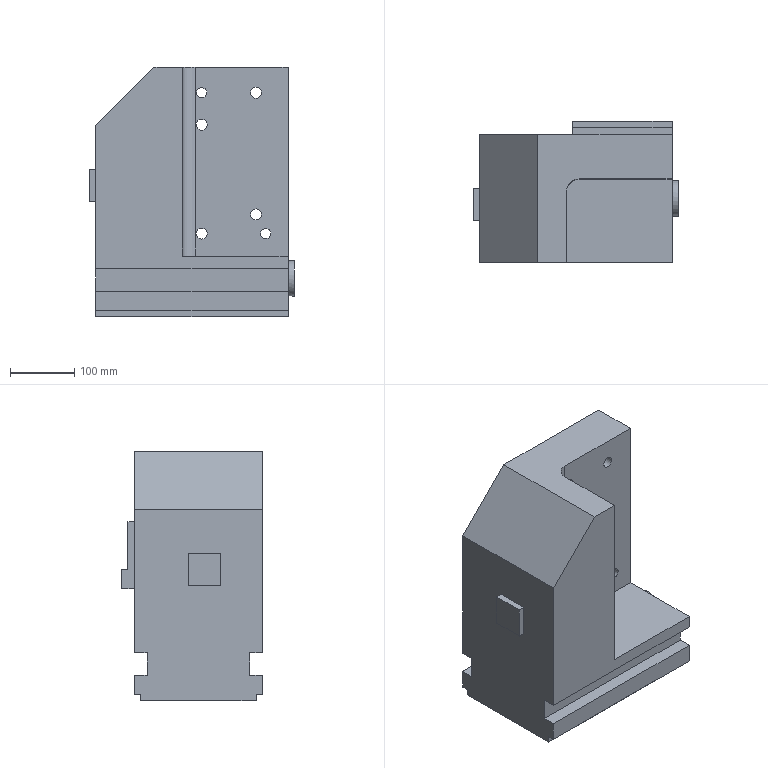Part | NX | features solid 2 | 1 solid | 50 faces | box 320 x 220 x 390 mm | volume 15914614 mm3 | plane 38 | cylinder 12 | commonest cylinder face diameters 17 x4 26 x4 16 x2 40 x1 55 x1
STEP:
#1=CARTESIAN_POINT('',(495.,1030.,-88.));
#2=VERTEX_POINT('',#1);
#3=CARTESIAN_POINT('',(495.,1030.,-75.));
#4=DIRECTION('',(0.,1.,0.));
#5=DIRECTION('',(0.,0.,-1.));
#6=AXIS2_PLACEMENT_3D('',#3,#4,#5);
#7=CIRCLE('',#6,13.);
#8=EDGE_CURVE('',#2,#2,#7,.T.);
#9=ORIENTED_EDGE('',*,*,#8,.F.);
#10=EDGE_LOOP('',(#9));
#11=FACE_BOUND('',#10,.T.);
#12=CARTESIAN_POINT('',(510.,1030.,-97.));
#13=VERTEX_POINT('',#12);
#14=CARTESIAN_POINT('',(510.,1030.,-105.));
#15=DIRECTION('',(0.,1.,0.));
#16=DIRECTION('',(0.,0.,1.));
#17=AXIS2_PLACEMENT_3D('',#14,#15,#16);
#18=CIRCLE('',#17,8.);
#19=EDGE_CURVE('',#13,#13,#18,.F.);
#20=ORIENTED_EDGE('',*,*,#19,.T.);
#21=EDGE_LOOP('',(#20));
#22=FACE_BOUND('',#21,.T.);
#23=CARTESIAN_POINT('',(410.,1030.,-92.));
#24=VERTEX_POINT('',#23);
#25=CARTESIAN_POINT('',(410.,1030.,-105.));
#26=DIRECTION('',(0.,1.,0.));
#27=DIRECTION('',(0.,0.,1.));
#28=AXIS2_PLACEMENT_3D('',#25,#26,#27);
#29=CIRCLE('',#28,13.);
#30=EDGE_CURVE('',#24,#24,#29,.F.);
#31=ORIENTED_EDGE('',*,*,#30,.T.);
#32=EDGE_LOOP('',(#31));
#33=FACE_BOUND('',#32,.T.);
#34=CARTESIAN_POINT('',(495.,1030.,128.));
#35=VERTEX_POINT('',#34);
#36=CARTESIAN_POINT('',(495.,1030.,115.));
#37=DIRECTION('',(0.,1.,0.));
#38=DIRECTION('',(0.,0.,1.));
#39=AXIS2_PLACEMENT_3D('',#36,#37,#38);
#40=CIRCLE('',#39,13.);
#41=EDGE_CURVE('',#35,#35,#40,.F.);
#42=ORIENTED_EDGE('',*,*,#41,.T.);
#43=EDGE_LOOP('',(#42));
#44=FACE_BOUND('',#43,.T.);
#45=CARTESIAN_POINT('',(410.,1030.,123.));
#46=VERTEX_POINT('',#45);
#47=CARTESIAN_POINT('',(410.,1030.,115.));
#48=DIRECTION('',(0.,1.,0.));
#49=DIRECTION('',(0.,0.,1.));
#50=AXIS2_PLACEMENT_3D('',#47,#48,#49);
#51=CIRCLE('',#50,8.);
#52=EDGE_CURVE('',#46,#46,#51,.F.);
#53=ORIENTED_EDGE('',*,*,#52,.T.);
#54=EDGE_LOOP('',(#53));
#55=FACE_BOUND('',#54,.T.);
#56=CARTESIAN_POINT('',(410.,1030.,78.));
#57=VERTEX_POINT('',#56);
#58=CARTESIAN_POINT('',(410.,1030.,65.));
#59=DIRECTION('',(0.,1.,0.));
#60=DIRECTION('',(0.,0.,1.));
#61=AXIS2_PLACEMENT_3D('',#58,#59,#60);
#62=CIRCLE('',#61,13.);
#63=EDGE_CURVE('',#57,#57,#62,.F.);
#64=ORIENTED_EDGE('',*,*,#63,.T.);
#65=EDGE_LOOP('',(#64));
#66=FACE_BOUND('',#65,.T.);
#67=CARTESIAN_POINT('',(390.,1030.,-60.));
#68=VERTEX_POINT('',#67);
#69=CARTESIAN_POINT('',(390.,1030.,45.));
#70=VERTEX_POINT('',#69);
#71=CARTESIAN_POINT('',(390.,1030.,-319.092));
#72=DIRECTION('',(0.,0.,1.));
#73=VECTOR('',#72,1000.);
#74=LINE('',#71,#73);
#75=EDGE_CURVE('',#68,#70,#74,.T.);
#76=ORIENTED_EDGE('',*,*,#75,.F.);
#77=CARTESIAN_POINT('',(545.,1030.,-60.));
#78=VERTEX_POINT('',#77);
#79=CARTESIAN_POINT('',(390.,1030.,-60.));
#80=DIRECTION('',(1.,0.,0.));
#81=VECTOR('',#80,1000.);
#82=LINE('',#79,#81);
#83=EDGE_CURVE('',#68,#78,#82,.T.);
#84=ORIENTED_EDGE('',*,*,#83,.T.);
#85=CARTESIAN_POINT('',(545.,1030.,-160.));
#86=VERTEX_POINT('',#85);
#87=CARTESIAN_POINT('',(545.,1030.,-319.092));
#88=DIRECTION('',(0.,0.,-1.));
#89=VECTOR('',#88,1000.);
#90=LINE('',#87,#89);
#91=EDGE_CURVE('',#86,#78,#90,.F.);
#92=ORIENTED_EDGE('',*,*,#91,.F.);
#93=CARTESIAN_POINT('',(245.,1030.,-160.));
#94=VERTEX_POINT('',#93);
#95=CARTESIAN_POINT('',(319.092,1030.,-160.));
#96=DIRECTION('',(1.,0.,0.));
#97=VECTOR('',#96,1000.);
#98=LINE('',#95,#97);
#99=EDGE_CURVE('',#94,#86,#98,.T.);
#100=ORIENTED_EDGE('',*,*,#99,.F.);
#101=CARTESIAN_POINT('',(245.,1030.,64.411));
#102=VERTEX_POINT('',#101);
#103=CARTESIAN_POINT('',(245.,1030.,0.));
#104=DIRECTION('',(0.,0.,1.));
#105=VECTOR('',#104,1000.);
#106=LINE('',#103,#105);
#107=EDGE_CURVE('',#94,#102,#106,.T.);
#108=ORIENTED_EDGE('',*,*,#107,.T.);
#109=CARTESIAN_POINT('',(335.589,1030.,155.));
#110=VERTEX_POINT('',#109);
#111=CARTESIAN_POINT('',(90.294,1030.,-90.294));
#112=DIRECTION('',(0.7071,0.,0.7071));
#113=VECTOR('',#112,1000.);
#114=LINE('',#111,#113);
#115=EDGE_CURVE('',#102,#110,#114,.T.);
#116=ORIENTED_EDGE('',*,*,#115,.T.);
#117=CARTESIAN_POINT('',(545.,1030.,155.));
#118=VERTEX_POINT('',#117);
#119=CARTESIAN_POINT('',(319.092,1030.,155.));
#120=DIRECTION('',(1.,0.,0.));
#121=VECTOR('',#120,1000.);
#122=LINE('',#119,#121);
#123=EDGE_CURVE('',#110,#118,#122,.T.);
#124=ORIENTED_EDGE('',*,*,#123,.T.);
#125=CARTESIAN_POINT('',(545.,1030.,45.));
#126=VERTEX_POINT('',#125);
#127=CARTESIAN_POINT('',(545.,1030.,-319.092));
#128=DIRECTION('',(0.,0.,-1.));
#129=VECTOR('',#128,1000.);
#130=LINE('',#127,#129);
#131=EDGE_CURVE('',#126,#118,#130,.F.);
#132=ORIENTED_EDGE('',*,*,#131,.F.);
#133=CARTESIAN_POINT('',(390.,1030.,45.));
#134=DIRECTION('',(1.,0.,0.));
#135=VECTOR('',#134,1000.);
#136=LINE('',#133,#135);
#137=EDGE_CURVE('',#70,#126,#136,.T.);
#138=ORIENTED_EDGE('',*,*,#137,.F.);
#139=EDGE_LOOP('',(#76,#84,#92,#100,#108,#116,#124,#132,#138));
#140=FACE_BOUND('',#139,.T.);
#141=CARTESIAN_POINT('',(319.092,1030.,-319.092));
#142=DIRECTION('',(0.,1.,0.));
#143=DIRECTION('',(0.,0.,1.));
#144=AXIS2_PLACEMENT_3D('',#141,#142,#143);
#145=PLANE('',#144);
#146=ADVANCED_FACE('',(#11,#22,#33,#44,#55,#66,#140),#145,.T.);
#147=CARTESIAN_POINT('',(245.,1030.,-225.));
#148=VERTEX_POINT('',#147);
#149=CARTESIAN_POINT('',(245.,1030.,-195.));
#150=VERTEX_POINT('',#149);
#151=CARTESIAN_POINT('',(245.,1030.,0.));
#152=DIRECTION('',(0.,0.,1.));
#153=VECTOR('',#152,1000.);
#154=LINE('',#151,#153);
#155=EDGE_CURVE('',#148,#150,#154,.T.);
#156=ORIENTED_EDGE('',*,*,#155,.T.);
#157=CARTESIAN_POINT('',(545.,1030.,-195.));
#158=VERTEX_POINT('',#157);
#159=CARTESIAN_POINT('',(319.092,1030.,-195.));
#160=DIRECTION('',(1.,0.,0.));
#161=VECTOR('',#160,1000.);
#162=LINE('',#159,#161);
#163=EDGE_CURVE('',#150,#158,#162,.T.);
#164=ORIENTED_EDGE('',*,*,#163,.T.);
#165=CARTESIAN_POINT('',(545.,1030.,-225.));
#166=VERTEX_POINT('',#165);
#167=CARTESIAN_POINT('',(545.,1030.,-319.092));
#168=DIRECTION('',(0.,0.,-1.));
#169=VECTOR('',#168,1000.);
#170=LINE('',#167,#169);
#171=EDGE_CURVE('',#166,#158,#170,.F.);
#172=ORIENTED_EDGE('',*,*,#171,.F.);
#173=CARTESIAN_POINT('',(245.,1030.,-225.));
#174=DIRECTION('',(1.,0.,0.));
#175=VECTOR('',#174,1000.);
#176=LINE('',#173,#175);
#177=EDGE_CURVE('',#148,#166,#176,.T.);
#178=ORIENTED_EDGE('',*,*,#177,.F.);
#179=EDGE_LOOP('',(#156,#164,#172,#178));
#180=FACE_BOUND('',#179,.T.);
#181=CARTESIAN_POINT('',(319.092,1030.,-319.092));
#182=DIRECTION('',(0.,1.,0.));
#183=DIRECTION('',(0.,0.,1.));
#184=AXIS2_PLACEMENT_3D('',#181,#182,#183);
#185=PLANE('',#184);
#186=ADVANCED_FACE('',(#180),#185,.T.);
#187=CARTESIAN_POINT('',(495.,960.,-83.5));
#188=VERTEX_POINT('',#187);
#189=CARTESIAN_POINT('',(495.,960.,-75.));
#190=DIRECTION('',(0.,-1.,0.));
#191=DIRECTION('',(0.,0.,-1.));
#192=AXIS2_PLACEMENT_3D('',#189,#190,#191);
#193=CIRCLE('',#192,8.5);
#194=EDGE_CURVE('',#188,#188,#193,.T.);
#195=ORIENTED_EDGE('',*,*,#194,.F.);
#196=EDGE_LOOP('',(#195));
#197=FACE_BOUND('',#196,.T.);
#198=CARTESIAN_POINT('',(410.,960.,56.5));
#199=VERTEX_POINT('',#198);
#200=CARTESIAN_POINT('',(410.,960.,65.));
#201=DIRECTION('',(0.,-1.,0.));
#202=DIRECTION('',(0.,0.,-1.));
#203=AXIS2_PLACEMENT_3D('',#200,#201,#202);
#204=CIRCLE('',#203,8.5);
#205=EDGE_CURVE('',#199,#199,#204,.T.);
#206=ORIENTED_EDGE('',*,*,#205,.F.);
#207=EDGE_LOOP('',(#206));
#208=FACE_BOUND('',#207,.T.);
#209=CARTESIAN_POINT('',(510.,960.,-113.));
#210=VERTEX_POINT('',#209);
#211=CARTESIAN_POINT('',(510.,960.,-105.));
#212=DIRECTION('',(0.,-1.,0.));
#213=DIRECTION('',(0.,0.,-1.));
#214=AXIS2_PLACEMENT_3D('',#211,#212,#213);
#215=CIRCLE('',#214,8.);
#216=EDGE_CURVE('',#210,#210,#215,.T.);
#217=ORIENTED_EDGE('',*,*,#216,.F.);
#218=EDGE_LOOP('',(#217));
#219=FACE_BOUND('',#218,.T.);
#220=CARTESIAN_POINT('',(410.,960.,-113.5));
#221=VERTEX_POINT('',#220);
#222=CARTESIAN_POINT('',(410.,960.,-105.));
#223=DIRECTION('',(0.,-1.,0.));
#224=DIRECTION('',(0.,0.,-1.));
#225=AXIS2_PLACEMENT_3D('',#222,#223,#224);
#226=CIRCLE('',#225,8.5);
#227=EDGE_CURVE('',#221,#221,#226,.T.);
#228=ORIENTED_EDGE('',*,*,#227,.F.);
#229=EDGE_LOOP('',(#228));
#230=FACE_BOUND('',#229,.T.);
#231=CARTESIAN_POINT('',(545.,960.,-140.));
#232=VERTEX_POINT('',#231);
#233=CARTESIAN_POINT('',(545.,960.,155.));
#234=VERTEX_POINT('',#233);
#235=CARTESIAN_POINT('',(545.,960.,-180.));
#236=DIRECTION('',(0.,0.,-1.));
#237=VECTOR('',#236,1000.);
#238=LINE('',#235,#237);
#239=EDGE_CURVE('',#232,#234,#238,.F.);
#240=ORIENTED_EDGE('',*,*,#239,.T.);
#241=CARTESIAN_POINT('',(400.,960.,155.));
#242=VERTEX_POINT('',#241);
#243=CARTESIAN_POINT('',(472.326,960.,155.));
#244=DIRECTION('',(-1.,0.,0.));
#245=VECTOR('',#244,1000.);
#246=LINE('',#243,#245);
#247=EDGE_CURVE('',#234,#242,#246,.T.);
#248=ORIENTED_EDGE('',*,*,#247,.T.);
#249=CARTESIAN_POINT('',(400.,960.,-140.));
#250=VERTEX_POINT('',#249);
#251=CARTESIAN_POINT('',(400.,960.,-180.));
#252=DIRECTION('',(0.,0.,-1.));
#253=VECTOR('',#252,1000.);
#254=LINE('',#251,#253);
#255=EDGE_CURVE('',#242,#250,#254,.T.);
#256=ORIENTED_EDGE('',*,*,#255,.T.);
#257=CARTESIAN_POINT('',(785.,960.,-140.));
#258=DIRECTION('',(-1.,0.,0.));
#259=VECTOR('',#258,1000.);
#260=LINE('',#257,#259);
#261=EDGE_CURVE('',#250,#232,#260,.F.);
#262=ORIENTED_EDGE('',*,*,#261,.T.);
#263=EDGE_LOOP('',(#240,#248,#256,#262));
#264=FACE_BOUND('',#263,.T.);
#265=CARTESIAN_POINT('',(410.,960.,107.));
#266=VERTEX_POINT('',#265);
#267=CARTESIAN_POINT('',(410.,960.,115.));
#268=DIRECTION('',(0.,-1.,0.));
#269=DIRECTION('',(0.,0.,-1.));
#270=AXIS2_PLACEMENT_3D('',#267,#268,#269);
#271=CIRCLE('',#270,8.);
#272=EDGE_CURVE('',#266,#266,#271,.T.);
#273=ORIENTED_EDGE('',*,*,#272,.F.);
#274=EDGE_LOOP('',(#273));
#275=FACE_BOUND('',#274,.T.);
#276=CARTESIAN_POINT('',(495.,960.,106.5));
#277=VERTEX_POINT('',#276);
#278=CARTESIAN_POINT('',(495.,960.,115.));
#279=DIRECTION('',(0.,-1.,0.));
#280=DIRECTION('',(0.,0.,-1.));
#281=AXIS2_PLACEMENT_3D('',#278,#279,#280);
#282=CIRCLE('',#281,8.5);
#283=EDGE_CURVE('',#277,#277,#282,.T.);
#284=ORIENTED_EDGE('',*,*,#283,.F.);
#285=EDGE_LOOP('',(#284));
#286=FACE_BOUND('',#285,.T.);
#287=CARTESIAN_POINT('',(645.,960.,-180.));
#288=DIRECTION('',(0.,1.,0.));
#289=DIRECTION('',(0.,0.,1.));
#290=AXIS2_PLACEMENT_3D('',#287,#288,#289);
#291=PLANE('',#290);
#292=ADVANCED_FACE('',(#197,#208,#219,#230,#264,#275,#286),#291,.F.);
#293=ORIENTED_EDGE('',*,*,#91,.T.);
#294=CARTESIAN_POINT('',(545.,1050.,-60.));
#295=VERTEX_POINT('',#294);
#296=CARTESIAN_POINT('',(545.,1030.,-60.));
#297=DIRECTION('',(0.,1.,0.));
#298=VECTOR('',#297,1000.);
#299=LINE('',#296,#298);
#300=EDGE_CURVE('',#78,#295,#299,.T.);
#301=ORIENTED_EDGE('',*,*,#300,.T.);
#302=CARTESIAN_POINT('',(545.,1050.,-30.));
#303=VERTEX_POINT('',#302);
#304=CARTESIAN_POINT('',(545.,1050.,-30.));
#305=DIRECTION('',(0.,0.,1.));
#306=VECTOR('',#305,1000.);
#307=LINE('',#304,#306);
#308=EDGE_CURVE('',#303,#295,#307,.F.);
#309=ORIENTED_EDGE('',*,*,#308,.F.);
#310=CARTESIAN_POINT('',(545.,1040.,-30.));
#311=VERTEX_POINT('',#310);
#312=CARTESIAN_POINT('',(545.,1030.,-30.));
#313=DIRECTION('',(0.,1.,0.));
#314=VECTOR('',#313,1000.);
#315=LINE('',#312,#314);
#316=EDGE_CURVE('',#311,#303,#315,.T.);
#317=ORIENTED_EDGE('',*,*,#316,.F.);
#318=CARTESIAN_POINT('',(545.,1040.,45.));
#319=VERTEX_POINT('',#318);
#320=CARTESIAN_POINT('',(545.,1040.,7.5));
#321=DIRECTION('',(0.,0.,1.));
#322=VECTOR('',#321,1000.);
#323=LINE('',#320,#322);
#324=EDGE_CURVE('',#311,#319,#323,.T.);
#325=ORIENTED_EDGE('',*,*,#324,.T.);
#326=CARTESIAN_POINT('',(545.,1035.,45.));
#327=DIRECTION('',(0.,-1.,0.));
#328=VECTOR('',#327,1000.);
#329=LINE('',#326,#328);
#330=EDGE_CURVE('',#319,#126,#329,.T.);
#331=ORIENTED_EDGE('',*,*,#330,.T.);
#332=ORIENTED_EDGE('',*,*,#131,.T.);
#333=CARTESIAN_POINT('',(545.,965.,155.));
#334=DIRECTION('',(0.,-1.,0.));
#335=VECTOR('',#334,1000.);
#336=LINE('',#333,#335);
#337=EDGE_CURVE('',#234,#118,#336,.F.);
#338=ORIENTED_EDGE('',*,*,#337,.F.);
#339=ORIENTED_EDGE('',*,*,#239,.F.);
#340=CARTESIAN_POINT('',(545.,830.,-140.));
#341=VERTEX_POINT('',#340);
#342=CARTESIAN_POINT('',(545.,965.,-140.));
#343=DIRECTION('',(0.,-1.,0.));
#344=VECTOR('',#343,1000.);
#345=LINE('',#342,#344);
#346=EDGE_CURVE('',#232,#341,#345,.T.);
#347=ORIENTED_EDGE('',*,*,#346,.T.);
#348=CARTESIAN_POINT('',(545.,830.,-160.));
#349=VERTEX_POINT('',#348);
#350=CARTESIAN_POINT('',(545.,830.,87.071));
#351=DIRECTION('',(0.,0.,1.));
#352=VECTOR('',#351,1000.);
#353=LINE('',#350,#352);
#354=EDGE_CURVE('',#341,#349,#353,.F.);
#355=ORIENTED_EDGE('',*,*,#354,.T.);
#356=CARTESIAN_POINT('',(545.,850.,-160.));
#357=VERTEX_POINT('',#356);
#358=CARTESIAN_POINT('',(545.,766.,-160.));
#359=DIRECTION('',(0.,-1.,0.));
#360=VECTOR('',#359,1000.);
#361=LINE('',#358,#360);
#362=EDGE_CURVE('',#357,#349,#361,.T.);
#363=ORIENTED_EDGE('',*,*,#362,.F.);
#364=CARTESIAN_POINT('',(545.,850.,-195.));
#365=VERTEX_POINT('',#364);
#366=CARTESIAN_POINT('',(545.,850.,-10.));
#367=DIRECTION('',(0.,0.,-1.));
#368=VECTOR('',#367,1000.);
#369=LINE('',#366,#368);
#370=EDGE_CURVE('',#365,#357,#369,.F.);
#371=ORIENTED_EDGE('',*,*,#370,.F.);
#372=CARTESIAN_POINT('',(545.,830.,-195.));
#373=VERTEX_POINT('',#372);
#374=CARTESIAN_POINT('',(545.,766.,-195.));
#375=DIRECTION('',(0.,-1.,0.));
#376=VECTOR('',#375,1000.);
#377=LINE('',#374,#376);
#378=EDGE_CURVE('',#365,#373,#377,.T.);
#379=ORIENTED_EDGE('',*,*,#378,.T.);
#380=CARTESIAN_POINT('',(545.,830.,-225.));
#381=VERTEX_POINT('',#380);
#382=CARTESIAN_POINT('',(545.,830.,87.071));
#383=DIRECTION('',(0.,0.,1.));
#384=VECTOR('',#383,1000.);
#385=LINE('',#382,#384);
#386=EDGE_CURVE('',#373,#381,#385,.F.);
#387=ORIENTED_EDGE('',*,*,#386,.T.);
#388=CARTESIAN_POINT('',(545.,840.,-225.));
#389=VERTEX_POINT('',#388);
#390=CARTESIAN_POINT('',(545.,830.,-225.));
#391=DIRECTION('',(0.,-1.,0.));
#392=VECTOR('',#391,1000.);
#393=LINE('',#390,#392);
#394=EDGE_CURVE('',#381,#389,#393,.F.);
#395=ORIENTED_EDGE('',*,*,#394,.T.);
#396=CARTESIAN_POINT('',(545.,840.,-235.));
#397=VERTEX_POINT('',#396);
#398=CARTESIAN_POINT('',(545.,840.,-235.));
#399=DIRECTION('',(0.,0.,-1.));
#400=VECTOR('',#399,1000.);
#401=LINE('',#398,#400);
#402=EDGE_CURVE('',#397,#389,#401,.F.);
#403=ORIENTED_EDGE('',*,*,#402,.F.);
#404=CARTESIAN_POINT('',(545.,1020.,-235.));
#405=VERTEX_POINT('',#404);
#406=CARTESIAN_POINT('',(545.,1020.,-235.));
#407=DIRECTION('',(0.,-1.,0.));
#408=VECTOR('',#407,1000.);
#409=LINE('',#406,#408);
#410=EDGE_CURVE('',#397,#405,#409,.F.);
#411=ORIENTED_EDGE('',*,*,#410,.T.);
#412=CARTESIAN_POINT('',(545.,1020.,-225.));
#413=VERTEX_POINT('',#412);
#414=CARTESIAN_POINT('',(545.,1020.,-235.));
#415=DIRECTION('',(0.,0.,-1.));
#416=VECTOR('',#415,1000.);
#417=LINE('',#414,#416);
#418=EDGE_CURVE('',#405,#413,#417,.F.);
#419=ORIENTED_EDGE('',*,*,#418,.T.);
#420=CARTESIAN_POINT('',(545.,1030.,-225.));
#421=DIRECTION('',(0.,-1.,0.));
#422=VECTOR('',#421,1000.);
#423=LINE('',#420,#422);
#424=EDGE_CURVE('',#166,#413,#423,.T.);
#425=ORIENTED_EDGE('',*,*,#424,.F.);
#426=ORIENTED_EDGE('',*,*,#171,.T.);
#427=CARTESIAN_POINT('',(545.,1010.,-195.));
#428=VERTEX_POINT('',#427);
#429=CARTESIAN_POINT('',(545.,1040.,-195.));
#430=DIRECTION('',(0.,-1.,0.));
#431=VECTOR('',#430,1000.);
#432=LINE('',#429,#431);
#433=EDGE_CURVE('',#158,#428,#432,.T.);
#434=ORIENTED_EDGE('',*,*,#433,.T.);
#435=CARTESIAN_POINT('',(545.,1010.,-160.));
#436=VERTEX_POINT('',#435);
#437=CARTESIAN_POINT('',(545.,1010.,-10.));
#438=DIRECTION('',(0.,0.,-1.));
#439=VECTOR('',#438,1000.);
#440=LINE('',#437,#439);
#441=EDGE_CURVE('',#428,#436,#440,.F.);
#442=ORIENTED_EDGE('',*,*,#441,.T.);
#443=CARTESIAN_POINT('',(545.,1040.,-160.));
#444=DIRECTION('',(0.,-1.,0.));
#445=VECTOR('',#444,1000.);
#446=LINE('',#443,#445);
#447=EDGE_CURVE('',#86,#436,#446,.T.);
#448=ORIENTED_EDGE('',*,*,#447,.F.);
#449=EDGE_LOOP('',(#293,#301,#309,#317,#325,#331,#332,#338,#339,#347,#355,#363,#371,#379,#387,#395,#403,#411,#419,#425,#426,#434,#442,#448));
#450=FACE_BOUND('',#449,.T.);
#451=CARTESIAN_POINT('',(545.,957.5,-175.));
#452=VERTEX_POINT('',#451);
#453=CARTESIAN_POINT('',(545.,930.,-175.));
#454=DIRECTION('',(1.,0.,0.));
#455=DIRECTION('',(0.,1.,0.));
#456=AXIS2_PLACEMENT_3D('',#453,#454,#455);
#457=CIRCLE('',#456,27.5);
#458=EDGE_CURVE('',#452,#452,#457,.T.);
#459=ORIENTED_EDGE('',*,*,#458,.F.);
#460=EDGE_LOOP('',(#459));
#461=FACE_BOUND('',#460,.T.);
#462=CARTESIAN_POINT('',(545.,965.,-10.));
#463=DIRECTION('',(1.,0.,0.));
#464=DIRECTION('',(0.,1.,0.));
#465=AXIS2_PLACEMENT_3D('',#462,#463,#464);
#466=PLANE('',#465);
#467=ADVANCED_FACE('',(#450,#461),#466,.T.);
#468=CARTESIAN_POINT('',(245.,1010.,-160.));
#469=VERTEX_POINT('',#468);
#470=CARTESIAN_POINT('',(245.,1040.,-160.));
#471=DIRECTION('',(0.,-1.,0.));
#472=VECTOR('',#471,1000.);
#473=LINE('',#470,#472);
#474=EDGE_CURVE('',#94,#469,#473,.T.);
#475=ORIENTED_EDGE('',*,*,#474,.T.);
#476=CARTESIAN_POINT('',(245.,1010.,-195.));
#477=VERTEX_POINT('',#476);
#478=CARTESIAN_POINT('',(245.,1010.,0.));
#479=DIRECTION('',(0.,0.,1.));
#480=VECTOR('',#479,1000.);
#481=LINE('',#478,#480);
#482=EDGE_CURVE('',#477,#469,#481,.T.);
#483=ORIENTED_EDGE('',*,*,#482,.F.);
#484=CARTESIAN_POINT('',(245.,1040.,-195.));
#485=DIRECTION('',(0.,-1.,0.));
#486=VECTOR('',#485,1000.);
#487=LINE('',#484,#486);
#488=EDGE_CURVE('',#150,#477,#487,.T.);
#489=ORIENTED_EDGE('',*,*,#488,.F.);
#490=ORIENTED_EDGE('',*,*,#155,.F.);
#491=CARTESIAN_POINT('',(245.,1020.,-225.));
#492=VERTEX_POINT('',#491);
#493=CARTESIAN_POINT('',(245.,1030.,-225.));
#494=DIRECTION('',(0.,-1.,0.));
#495=VECTOR('',#494,1000.);
#496=LINE('',#493,#495);
#497=EDGE_CURVE('',#148,#492,#496,.T.);
#498=ORIENTED_EDGE('',*,*,#497,.T.);
#499=CARTESIAN_POINT('',(245.,1020.,-235.));
#500=VERTEX_POINT('',#499);
#501=CARTESIAN_POINT('',(245.,1020.,-235.));
#502=DIRECTION('',(0.,0.,-1.));
#503=VECTOR('',#502,1000.);
#504=LINE('',#501,#503);
#505=EDGE_CURVE('',#500,#492,#504,.F.);
#506=ORIENTED_EDGE('',*,*,#505,.F.);
#507=CARTESIAN_POINT('',(245.,840.,-235.));
#508=VERTEX_POINT('',#507);
#509=CARTESIAN_POINT('',(245.,1020.,-235.));
#510=DIRECTION('',(0.,-1.,0.));
#511=VECTOR('',#510,1000.);
#512=LINE('',#509,#511);
#513=EDGE_CURVE('',#508,#500,#512,.F.);
#514=ORIENTED_EDGE('',*,*,#513,.F.);
#515=CARTESIAN_POINT('',(245.,840.,-225.));
#516=VERTEX_POINT('',#515);
#517=CARTESIAN_POINT('',(245.,840.,-235.));
#518=DIRECTION('',(0.,0.,-1.));
#519=VECTOR('',#518,1000.);
#520=LINE('',#517,#519);
#521=EDGE_CURVE('',#508,#516,#520,.F.);
#522=ORIENTED_EDGE('',*,*,#521,.T.);
#523=CARTESIAN_POINT('',(245.,830.,-225.));
#524=VERTEX_POINT('',#523);
#525=CARTESIAN_POINT('',(245.,830.,-225.));
#526=DIRECTION('',(0.,-1.,0.));
#527=VECTOR('',#526,1000.);
#528=LINE('',#525,#527);
#529=EDGE_CURVE('',#524,#516,#528,.F.);
#530=ORIENTED_EDGE('',*,*,#529,.F.);
#531=CARTESIAN_POINT('',(245.,830.,-195.));
#532=VERTEX_POINT('',#531);
#533=CARTESIAN_POINT('',(245.,830.,0.));
#534=DIRECTION('',(0.,0.,1.));
#535=VECTOR('',#534,1000.);
#536=LINE('',#533,#535);
#537=EDGE_CURVE('',#524,#532,#536,.T.);
#538=ORIENTED_EDGE('',*,*,#537,.T.);
#539=CARTESIAN_POINT('',(245.,850.,-195.));
#540=VERTEX_POINT('',#539);
#541=CARTESIAN_POINT('',(245.,766.,-195.));
#542=DIRECTION('',(0.,1.,0.));
#543=VECTOR('',#542,1000.);
#544=LINE('',#541,#543);
#545=EDGE_CURVE('',#532,#540,#544,.T.);
#546=ORIENTED_EDGE('',*,*,#545,.T.);
#547=CARTESIAN_POINT('',(245.,850.,-160.));
#548=VERTEX_POINT('',#547);
#549=CARTESIAN_POINT('',(245.,850.,0.));
#550=DIRECTION('',(0.,0.,1.));
#551=VECTOR('',#550,1000.);
#552=LINE('',#549,#551);
#553=EDGE_CURVE('',#540,#548,#552,.T.);
#554=ORIENTED_EDGE('',*,*,#553,.T.);
#555=CARTESIAN_POINT('',(245.,830.,-160.));
#556=VERTEX_POINT('',#555);
#557=CARTESIAN_POINT('',(245.,766.,-160.));
#558=DIRECTION('',(0.,1.,0.));
#559=VECTOR('',#558,1000.);
#560=LINE('',#557,#559);
#561=EDGE_CURVE('',#556,#548,#560,.T.);
#562=ORIENTED_EDGE('',*,*,#561,.F.);
#563=CARTESIAN_POINT('',(245.,830.,64.411));
#564=VERTEX_POINT('',#563);
#565=CARTESIAN_POINT('',(245.,830.,0.));
#566=DIRECTION('',(0.,0.,1.));
#567=VECTOR('',#566,1000.);
#568=LINE('',#565,#567);
#569=EDGE_CURVE('',#556,#564,#568,.T.);
#570=ORIENTED_EDGE('',*,*,#569,.T.);
#571=CARTESIAN_POINT('',(245.,0.,64.411));
#572=DIRECTION('',(0.,1.,0.));
#573=VECTOR('',#572,1000.);
#574=LINE('',#571,#573);
#575=EDGE_CURVE('',#564,#102,#574,.T.);
#576=ORIENTED_EDGE('',*,*,#575,.T.);
#577=ORIENTED_EDGE('',*,*,#107,.F.);
#578=EDGE_LOOP('',(#475,#483,#489,#490,#498,#506,#514,#522,#530,#538,#546,#554,#562,#570,#576,#577));
#579=FACE_BOUND('',#578,.T.);
#580=CARTESIAN_POINT('',(245.,895.,-55.));
#581=VERTEX_POINT('',#580);
#582=CARTESIAN_POINT('',(245.,945.,-55.));
#583=VERTEX_POINT('',#582);
#584=CARTESIAN_POINT('',(245.,895.,-55.));
#585=DIRECTION('',(0.,1.,0.));
#586=VECTOR('',#585,1000.);
#587=LINE('',#584,#586);
#588=EDGE_CURVE('',#581,#583,#587,.T.);
#589=ORIENTED_EDGE('',*,*,#588,.T.);
#590=CARTESIAN_POINT('',(245.,945.,-5.));
#591=VERTEX_POINT('',#590);
#592=CARTESIAN_POINT('',(245.,945.,-55.));
#593=DIRECTION('',(0.,0.,-1.));
#594=VECTOR('',#593,1000.);
#595=LINE('',#592,#594);
#596=EDGE_CURVE('',#583,#591,#595,.F.);
#597=ORIENTED_EDGE('',*,*,#596,.T.);
#598=CARTESIAN_POINT('',(245.,895.,-5.));
#599=VERTEX_POINT('',#598);
#600=CARTESIAN_POINT('',(245.,895.,-5.));
#601=DIRECTION('',(0.,-1.,0.));
#602=VECTOR('',#601,1000.);
#603=LINE('',#600,#602);
#604=EDGE_CURVE('',#599,#591,#603,.F.);
#605=ORIENTED_EDGE('',*,*,#604,.F.);
#606=CARTESIAN_POINT('',(245.,895.,-55.));
#607=DIRECTION('',(0.,0.,-1.));
#608=VECTOR('',#607,1000.);
#609=LINE('',#606,#608);
#610=EDGE_CURVE('',#581,#599,#609,.F.);
#611=ORIENTED_EDGE('',*,*,#610,.F.);
#612=EDGE_LOOP('',(#589,#597,#605,#611));
#613=FACE_BOUND('',#612,.T.);
#614=CARTESIAN_POINT('',(245.,0.,0.));
#615=DIRECTION('',(-1.,0.,0.));
#616=DIRECTION('',(0.,0.,-1.));
#617=AXIS2_PLACEMENT_3D('',#614,#615,#616);
#618=PLANE('',#617);
#619=ADVANCED_FACE('',(#579,#613),#618,.T.);
#620=ORIENTED_EDGE('',*,*,#386,.F.);
#621=CARTESIAN_POINT('',(725.255,830.,-195.));
#622=DIRECTION('',(-1.,0.,0.));
#623=VECTOR('',#622,1000.);
#624=LINE('',#621,#623);
#625=EDGE_CURVE('',#373,#532,#624,.T.);
#626=ORIENTED_EDGE('',*,*,#625,.T.);
#627=ORIENTED_EDGE('',*,*,#537,.F.);
#628=CARTESIAN_POINT('',(245.,830.,-225.));
#629=DIRECTION('',(1.,0.,0.));
#630=VECTOR('',#629,1000.);
#631=LINE('',#628,#630);
#632=EDGE_CURVE('',#524,#381,#631,.T.);
#633=ORIENTED_EDGE('',*,*,#632,.T.);
#634=EDGE_LOOP('',(#620,#626,#627,#633));
#635=FACE_BOUND('',#634,.T.);
#636=CARTESIAN_POINT('',(725.255,830.,87.071));
#637=DIRECTION('',(0.,-1.,0.));
#638=DIRECTION('',(0.,0.,-1.));
#639=AXIS2_PLACEMENT_3D('',#636,#637,#638);
#640=PLANE('',#639);
#641=ADVANCED_FACE('',(#635),#640,.T.);
#642=CARTESIAN_POINT('',(725.255,830.,-160.));
#643=DIRECTION('',(-1.,0.,0.));
#644=VECTOR('',#643,1000.);
#645=LINE('',#642,#644);
#646=EDGE_CURVE('',#349,#556,#645,.T.);
#647=ORIENTED_EDGE('',*,*,#646,.F.);
#648=ORIENTED_EDGE('',*,*,#354,.F.);
#649=CARTESIAN_POINT('',(380.,830.,-140.));
#650=VERTEX_POINT('',#649);
#651=CARTESIAN_POINT('',(785.,830.,-140.));
#652=DIRECTION('',(1.,0.,0.));
#653=VECTOR('',#652,1000.);
#654=LINE('',#651,#653);
#655=EDGE_CURVE('',#341,#650,#654,.F.);
#656=ORIENTED_EDGE('',*,*,#655,.T.);
#657=CARTESIAN_POINT('',(380.,830.,155.));
#658=VERTEX_POINT('',#657);
#659=CARTESIAN_POINT('',(380.,830.,-362.5));
#660=DIRECTION('',(0.,0.,-1.));
#661=VECTOR('',#660,1000.);
#662=LINE('',#659,#661);
#663=EDGE_CURVE('',#658,#650,#662,.T.);
#664=ORIENTED_EDGE('',*,*,#663,.F.);
#665=CARTESIAN_POINT('',(335.589,830.,155.));
#666=VERTEX_POINT('',#665);
#667=CARTESIAN_POINT('',(472.326,830.,155.));
#668=DIRECTION('',(1.,0.,0.));
#669=VECTOR('',#668,1000.);
#670=LINE('',#667,#669);
#671=EDGE_CURVE('',#666,#658,#670,.T.);
#672=ORIENTED_EDGE('',*,*,#671,.F.);
#673=CARTESIAN_POINT('',(496.458,830.,315.869));
#674=DIRECTION('',(-0.7071,0.,-0.7071));
#675=VECTOR('',#674,1000.);
#676=LINE('',#673,#675);
#677=EDGE_CURVE('',#666,#564,#676,.T.);
#678=ORIENTED_EDGE('',*,*,#677,.T.);
#679=ORIENTED_EDGE('',*,*,#569,.F.);
#680=EDGE_LOOP('',(#647,#648,#656,#664,#672,#678,#679));
#681=FACE_BOUND('',#680,.T.);
#682=CARTESIAN_POINT('',(725.255,830.,87.071));
#683=DIRECTION('',(0.,-1.,0.));
#684=DIRECTION('',(0.,0.,-1.));
#685=AXIS2_PLACEMENT_3D('',#682,#683,#684);
#686=PLANE('',#685);
#687=ADVANCED_FACE('',(#681),#686,.T.);
#688=ORIENTED_EDGE('',*,*,#410,.F.);
#689=CARTESIAN_POINT('',(245.,840.,-235.));
#690=DIRECTION('',(1.,0.,0.));
#691=VECTOR('',#690,1000.);
#692=LINE('',#689,#691);
#693=EDGE_CURVE('',#508,#397,#692,.T.);
#694=ORIENTED_EDGE('',*,*,#693,.F.);
#695=ORIENTED_EDGE('',*,*,#513,.T.);
#696=CARTESIAN_POINT('',(245.,1020.,-235.));
#697=DIRECTION('',(1.,0.,0.));
#698=VECTOR('',#697,1000.);
#699=LINE('',#696,#698);
#700=EDGE_CURVE('',#500,#405,#699,.T.);
#701=ORIENTED_EDGE('',*,*,#700,.T.);
#702=EDGE_LOOP('',(#688,#694,#695,#701));
#703=FACE_BOUND('',#702,.T.);
#704=CARTESIAN_POINT('',(327.674,1020.,-235.));
#705=DIRECTION('',(0.,0.,1.));
#706=DIRECTION('',(1.,0.,0.));
#707=AXIS2_PLACEMENT_3D('',#704,#705,#706);
#708=PLANE('',#707);
#709=ADVANCED_FACE('',(#703),#708,.F.);
#710=CARTESIAN_POINT('',(380.,940.,155.));
#711=VERTEX_POINT('',#710);
#712=CARTESIAN_POINT('',(400.,940.,155.));
#713=DIRECTION('',(0.,0.,1.));
#714=DIRECTION('',(0.,-1.,0.));
#715=AXIS2_PLACEMENT_3D('',#712,#713,#714);
#716=CIRCLE('',#715,20.);
#717=EDGE_CURVE('',#711,#242,#716,.F.);
#718=ORIENTED_EDGE('',*,*,#717,.F.);
#719=CARTESIAN_POINT('',(380.,940.,-140.));
#720=VERTEX_POINT('',#719);
#721=CARTESIAN_POINT('',(380.,940.,-362.5));
#722=DIRECTION('',(0.,0.,-1.));
#723=VECTOR('',#722,1000.);
#724=LINE('',#721,#723);
#725=EDGE_CURVE('',#720,#711,#724,.F.);
#726=ORIENTED_EDGE('',*,*,#725,.F.);
#727=CARTESIAN_POINT('',(400.,940.,-140.));
#728=DIRECTION('',(0.,0.,1.));
#729=DIRECTION('',(1.,0.,0.));
#730=AXIS2_PLACEMENT_3D('',#727,#728,#729);
#731=CIRCLE('',#730,20.);
#732=EDGE_CURVE('',#250,#720,#731,.T.);
#733=ORIENTED_EDGE('',*,*,#732,.F.);
#734=ORIENTED_EDGE('',*,*,#255,.F.);
#735=EDGE_LOOP('',(#718,#726,#733,#734));
#736=FACE_BOUND('',#735,.T.);
#737=CARTESIAN_POINT('',(400.,940.,-180.));
#738=DIRECTION('',(0.,0.,-1.));
#739=DIRECTION('',(0.,1.,0.));
#740=AXIS2_PLACEMENT_3D('',#737,#738,#739);
#741=CYLINDRICAL_SURFACE('',#740,20.);
#742=ADVANCED_FACE('',(#736),#741,.F.);
#743=CARTESIAN_POINT('',(380.,820.,-140.));
#744=DIRECTION('',(0.,1.,0.));
#745=VECTOR('',#744,1000.);
#746=LINE('',#743,#745);
#747=EDGE_CURVE('',#720,#650,#746,.F.);
#748=ORIENTED_EDGE('',*,*,#747,.F.);
#749=ORIENTED_EDGE('',*,*,#725,.T.);
#750=CARTESIAN_POINT('',(380.,820.,155.));
#751=DIRECTION('',(0.,-1.,0.));
#752=VECTOR('',#751,1000.);
#753=LINE('',#750,#752);
#754=EDGE_CURVE('',#711,#658,#753,.T.);
#755=ORIENTED_EDGE('',*,*,#754,.T.);
#756=ORIENTED_EDGE('',*,*,#663,.T.);
#757=EDGE_LOOP('',(#748,#749,#755,#756));
#758=FACE_BOUND('',#757,.T.);
#759=CARTESIAN_POINT('',(380.,820.,-362.5));
#760=DIRECTION('',(1.,0.,0.));
#761=DIRECTION('',(0.,1.,0.));
#762=AXIS2_PLACEMENT_3D('',#759,#760,#761);
#763=PLANE('',#762);
#764=ADVANCED_FACE('',(#758),#763,.T.);
#765=ORIENTED_EDGE('',*,*,#115,.F.);
#766=ORIENTED_EDGE('',*,*,#575,.F.);
#767=ORIENTED_EDGE('',*,*,#677,.F.);
#768=CARTESIAN_POINT('',(335.589,1020.,155.));
#769=DIRECTION('',(0.,-1.,0.));
#770=VECTOR('',#769,1000.);
#771=LINE('',#768,#770);
#772=EDGE_CURVE('',#110,#666,#771,.T.);
#773=ORIENTED_EDGE('',*,*,#772,.F.);
#774=EDGE_LOOP('',(#765,#766,#767,#773));
#775=FACE_BOUND('',#774,.T.);
#776=CARTESIAN_POINT('',(290.294,1020.,109.706));
#777=DIRECTION('',(-0.7071,0.,0.7071));
#778=DIRECTION('',(-0.7071,0.,-0.7071));
#779=AXIS2_PLACEMENT_3D('',#776,#777,#778);
#780=PLANE('',#779);
#781=ADVANCED_FACE('',(#775),#780,.T.);
#782=ORIENTED_EDGE('',*,*,#261,.F.);
#783=ORIENTED_EDGE('',*,*,#732,.T.);
#784=ORIENTED_EDGE('',*,*,#747,.T.);
#785=ORIENTED_EDGE('',*,*,#655,.F.);
#786=ORIENTED_EDGE('',*,*,#346,.F.);
#787=EDGE_LOOP('',(#782,#783,#784,#785,#786));
#788=FACE_BOUND('',#787,.T.);
#789=CARTESIAN_POINT('',(785.,820.,-140.));
#790=DIRECTION('',(0.,0.,1.));
#791=DIRECTION('',(0.,-1.,0.));
#792=AXIS2_PLACEMENT_3D('',#789,#790,#791);
#793=PLANE('',#792);
#794=ADVANCED_FACE('',(#788),#793,.T.);
#795=ORIENTED_EDGE('',*,*,#123,.F.);
#796=ORIENTED_EDGE('',*,*,#772,.T.);
#797=ORIENTED_EDGE('',*,*,#671,.T.);
#798=ORIENTED_EDGE('',*,*,#754,.F.);
#799=ORIENTED_EDGE('',*,*,#717,.T.);
#800=ORIENTED_EDGE('',*,*,#247,.F.);
#801=ORIENTED_EDGE('',*,*,#337,.T.);
#802=EDGE_LOOP('',(#795,#796,#797,#798,#799,#800,#801));
#803=FACE_BOUND('',#802,.T.);
#804=CARTESIAN_POINT('',(472.326,1020.,155.));
#805=DIRECTION('',(0.,0.,1.));
#806=DIRECTION('',(0.,-1.,0.));
#807=AXIS2_PLACEMENT_3D('',#804,#805,#806);
#808=PLANE('',#807);
#809=ADVANCED_FACE('',(#803),#808,.T.);
#810=ORIENTED_EDGE('',*,*,#497,.F.);
#811=ORIENTED_EDGE('',*,*,#177,.T.);
#812=ORIENTED_EDGE('',*,*,#424,.T.);
#813=CARTESIAN_POINT('',(245.,1020.,-225.));
#814=DIRECTION('',(1.,0.,0.));
#815=VECTOR('',#814,1000.);
#816=LINE('',#813,#815);
#817=EDGE_CURVE('',#492,#413,#816,.T.);
#818=ORIENTED_EDGE('',*,*,#817,.F.);
#819=EDGE_LOOP('',(#810,#811,#812,#818));
#820=FACE_BOUND('',#819,.T.);
#821=CARTESIAN_POINT('',(245.,1030.,-225.));
#822=DIRECTION('',(0.,0.,-1.));
#823=DIRECTION('',(1.,0.,0.));
#824=AXIS2_PLACEMENT_3D('',#821,#822,#823);
#825=PLANE('',#824);
#826=ADVANCED_FACE('',(#820),#825,.T.);
#827=ORIENTED_EDGE('',*,*,#817,.T.);
#828=ORIENTED_EDGE('',*,*,#418,.F.);
#829=ORIENTED_EDGE('',*,*,#700,.F.);
#830=ORIENTED_EDGE('',*,*,#505,.T.);
#831=EDGE_LOOP('',(#827,#828,#829,#830));
#832=FACE_BOUND('',#831,.T.);
#833=CARTESIAN_POINT('',(245.,1020.,-235.));
#834=DIRECTION('',(0.,-1.,0.));
#835=DIRECTION('',(0.,0.,-1.));
#836=AXIS2_PLACEMENT_3D('',#833,#834,#835);
#837=PLANE('',#836);
#838=ADVANCED_FACE('',(#832),#837,.F.);
#839=ORIENTED_EDGE('',*,*,#394,.F.);
#840=ORIENTED_EDGE('',*,*,#632,.F.);
#841=ORIENTED_EDGE('',*,*,#529,.T.);
#842=CARTESIAN_POINT('',(245.,840.,-225.));
#843=DIRECTION('',(1.,0.,0.));
#844=VECTOR('',#843,1000.);
#845=LINE('',#842,#844);
#846=EDGE_CURVE('',#516,#389,#845,.T.);
#847=ORIENTED_EDGE('',*,*,#846,.T.);
#848=EDGE_LOOP('',(#839,#840,#841,#847));
#849=FACE_BOUND('',#848,.T.);
#850=CARTESIAN_POINT('',(245.,830.,-225.));
#851=DIRECTION('',(0.,0.,-1.));
#852=DIRECTION('',(1.,0.,0.));
#853=AXIS2_PLACEMENT_3D('',#850,#851,#852);
#854=PLANE('',#853);
#855=ADVANCED_FACE('',(#849),#854,.T.);
#856=ORIENTED_EDGE('',*,*,#846,.F.);
#857=ORIENTED_EDGE('',*,*,#521,.F.);
#858=ORIENTED_EDGE('',*,*,#693,.T.);
#859=ORIENTED_EDGE('',*,*,#402,.T.);
#860=EDGE_LOOP('',(#856,#857,#858,#859));
#861=FACE_BOUND('',#860,.T.);
#862=CARTESIAN_POINT('',(245.,840.,-235.));
#863=DIRECTION('',(0.,-1.,0.));
#864=DIRECTION('',(0.,0.,-1.));
#865=AXIS2_PLACEMENT_3D('',#862,#863,#864);
#866=PLANE('',#865);
#867=ADVANCED_FACE('',(#861),#866,.T.);
#868=CARTESIAN_POINT('',(445.,850.,-160.));
#869=DIRECTION('',(1.,0.,0.));
#870=VECTOR('',#869,1000.);
#871=LINE('',#868,#870);
#872=EDGE_CURVE('',#548,#357,#871,.T.);
#873=ORIENTED_EDGE('',*,*,#872,.F.);
#874=ORIENTED_EDGE('',*,*,#553,.F.);
#875=CARTESIAN_POINT('',(445.,850.,-195.));
#876=DIRECTION('',(1.,0.,0.));
#877=VECTOR('',#876,1000.);
#878=LINE('',#875,#877);
#879=EDGE_CURVE('',#540,#365,#878,.T.);
#880=ORIENTED_EDGE('',*,*,#879,.T.);
#881=ORIENTED_EDGE('',*,*,#370,.T.);
#882=EDGE_LOOP('',(#873,#874,#880,#881));
#883=FACE_BOUND('',#882,.T.);
#884=CARTESIAN_POINT('',(445.,850.,-210.));
#885=DIRECTION('',(0.,-1.,0.));
#886=DIRECTION('',(0.,0.,-1.));
#887=AXIS2_PLACEMENT_3D('',#884,#885,#886);
#888=PLANE('',#887);
#889=ADVANCED_FACE('',(#883),#888,.T.);
#890=ORIENTED_EDGE('',*,*,#378,.F.);
#891=ORIENTED_EDGE('',*,*,#879,.F.);
#892=ORIENTED_EDGE('',*,*,#545,.F.);
#893=ORIENTED_EDGE('',*,*,#625,.F.);
#894=EDGE_LOOP('',(#890,#891,#892,#893));
#895=FACE_BOUND('',#894,.T.);
#896=CARTESIAN_POINT('',(445.,766.,-195.));
#897=DIRECTION('',(0.,0.,1.));
#898=DIRECTION('',(1.,0.,0.));
#899=AXIS2_PLACEMENT_3D('',#896,#897,#898);
#900=PLANE('',#899);
#901=ADVANCED_FACE('',(#895),#900,.T.);
#902=ORIENTED_EDGE('',*,*,#646,.T.);
#903=ORIENTED_EDGE('',*,*,#561,.T.);
#904=ORIENTED_EDGE('',*,*,#872,.T.);
#905=ORIENTED_EDGE('',*,*,#362,.T.);
#906=EDGE_LOOP('',(#902,#903,#904,#905));
#907=FACE_BOUND('',#906,.T.);
#908=CARTESIAN_POINT('',(445.,766.,-160.));
#909=DIRECTION('',(0.,0.,1.));
#910=DIRECTION('',(1.,0.,0.));
#911=AXIS2_PLACEMENT_3D('',#908,#909,#910);
#912=PLANE('',#911);
#913=ADVANCED_FACE('',(#907),#912,.F.);
#914=CARTESIAN_POINT('',(235.,945.,-55.));
#915=VERTEX_POINT('',#914);
#916=CARTESIAN_POINT('',(235.,945.,-5.));
#917=VERTEX_POINT('',#916);
#918=CARTESIAN_POINT('',(235.,945.,-55.));
#919=DIRECTION('',(0.,0.,-1.));
#920=VECTOR('',#919,1000.);
#921=LINE('',#918,#920);
#922=EDGE_CURVE('',#915,#917,#921,.F.);
#923=ORIENTED_EDGE('',*,*,#922,.T.);
#924=CARTESIAN_POINT('',(245.,945.,-5.));
#925=DIRECTION('',(-1.,0.,0.));
#926=VECTOR('',#925,1000.);
#927=LINE('',#924,#926);
#928=EDGE_CURVE('',#591,#917,#927,.T.);
#929=ORIENTED_EDGE('',*,*,#928,.F.);
#930=ORIENTED_EDGE('',*,*,#596,.F.);
#931=CARTESIAN_POINT('',(245.,945.,-55.));
#932=DIRECTION('',(-1.,0.,0.));
#933=VECTOR('',#932,1000.);
#934=LINE('',#931,#933);
#935=EDGE_CURVE('',#583,#915,#934,.T.);
#936=ORIENTED_EDGE('',*,*,#935,.T.);
#937=EDGE_LOOP('',(#923,#929,#930,#936));
#938=FACE_BOUND('',#937,.T.);
#939=CARTESIAN_POINT('',(245.,945.,-55.));
#940=DIRECTION('',(0.,-1.,0.));
#941=DIRECTION('',(0.,0.,-1.));
#942=AXIS2_PLACEMENT_3D('',#939,#940,#941);
#943=PLANE('',#942);
#944=ADVANCED_FACE('',(#938),#943,.F.);
#945=CARTESIAN_POINT('',(235.,895.,-55.));
#946=VERTEX_POINT('',#945);
#947=CARTESIAN_POINT('',(235.,895.,-55.));
#948=DIRECTION('',(0.,1.,0.));
#949=VECTOR('',#948,1000.);
#950=LINE('',#947,#949);
#951=EDGE_CURVE('',#946,#915,#950,.T.);
#952=ORIENTED_EDGE('',*,*,#951,.T.);
#953=ORIENTED_EDGE('',*,*,#935,.F.);
#954=ORIENTED_EDGE('',*,*,#588,.F.);
#955=CARTESIAN_POINT('',(245.,895.,-55.));
#956=DIRECTION('',(-1.,0.,0.));
#957=VECTOR('',#956,1000.);
#958=LINE('',#955,#957);
#959=EDGE_CURVE('',#581,#946,#958,.T.);
#960=ORIENTED_EDGE('',*,*,#959,.T.);
#961=EDGE_LOOP('',(#952,#953,#954,#960));
#962=FACE_BOUND('',#961,.T.);
#963=CARTESIAN_POINT('',(245.,895.,-55.));
#964=DIRECTION('',(0.,0.,1.));
#965=DIRECTION('',(0.,-1.,0.));
#966=AXIS2_PLACEMENT_3D('',#963,#964,#965);
#967=PLANE('',#966);
#968=ADVANCED_FACE('',(#962),#967,.F.);
#969=CARTESIAN_POINT('',(235.,895.,-5.));
#970=VERTEX_POINT('',#969);
#971=CARTESIAN_POINT('',(235.,895.,-55.));
#972=DIRECTION('',(0.,0.,-1.));
#973=VECTOR('',#972,1000.);
#974=LINE('',#971,#973);
#975=EDGE_CURVE('',#946,#970,#974,.F.);
#976=ORIENTED_EDGE('',*,*,#975,.F.);
#977=ORIENTED_EDGE('',*,*,#959,.F.);
#978=ORIENTED_EDGE('',*,*,#610,.T.);
#979=CARTESIAN_POINT('',(245.,895.,-5.));
#980=DIRECTION('',(-1.,0.,0.));
#981=VECTOR('',#980,1000.);
#982=LINE('',#979,#981);
#983=EDGE_CURVE('',#599,#970,#982,.T.);
#984=ORIENTED_EDGE('',*,*,#983,.T.);
#985=EDGE_LOOP('',(#976,#977,#978,#984));
#986=FACE_BOUND('',#985,.T.);
#987=CARTESIAN_POINT('',(245.,895.,-55.));
#988=DIRECTION('',(0.,-1.,0.));
#989=DIRECTION('',(0.,0.,-1.));
#990=AXIS2_PLACEMENT_3D('',#987,#988,#989);
#991=PLANE('',#990);
#992=ADVANCED_FACE('',(#986),#991,.T.);
#993=CARTESIAN_POINT('',(235.,895.,-5.));
#994=DIRECTION('',(0.,-1.,0.));
#995=VECTOR('',#994,1000.);
#996=LINE('',#993,#995);
#997=EDGE_CURVE('',#970,#917,#996,.F.);
#998=ORIENTED_EDGE('',*,*,#997,.F.);
#999=ORIENTED_EDGE('',*,*,#983,.F.);
#1000=ORIENTED_EDGE('',*,*,#604,.T.);
#1001=ORIENTED_EDGE('',*,*,#928,.T.);
#1002=EDGE_LOOP('',(#998,#999,#1000,#1001));
#1003=FACE_BOUND('',#1002,.T.);
#1004=CARTESIAN_POINT('',(245.,895.,-5.));
#1005=DIRECTION('',(0.,0.,1.));
#1006=DIRECTION('',(0.,-1.,0.));
#1007=AXIS2_PLACEMENT_3D('',#1004,#1005,#1006);
#1008=PLANE('',#1007);
#1009=ADVANCED_FACE('',(#1003),#1008,.T.);
#1010=ORIENTED_EDGE('',*,*,#922,.F.);
#1011=ORIENTED_EDGE('',*,*,#951,.F.);
#1012=ORIENTED_EDGE('',*,*,#975,.T.);
#1013=ORIENTED_EDGE('',*,*,#997,.T.);
#1014=EDGE_LOOP('',(#1010,#1011,#1012,#1013));
#1015=FACE_BOUND('',#1014,.T.);
#1016=CARTESIAN_POINT('',(235.,895.,-55.));
#1017=DIRECTION('',(1.,0.,0.));
#1018=DIRECTION('',(0.,1.,0.));
#1019=AXIS2_PLACEMENT_3D('',#1016,#1017,#1018);
#1020=PLANE('',#1019);
#1021=ADVANCED_FACE('',(#1015),#1020,.F.);
#1022=ORIENTED_EDGE('',*,*,#458,.T.);
#1023=EDGE_LOOP('',(#1022));
#1024=FACE_BOUND('',#1023,.T.);
#1025=CARTESIAN_POINT('',(555.,930.,-202.5));
#1026=VERTEX_POINT('',#1025);
#1027=CARTESIAN_POINT('',(555.,930.,-175.));
#1028=DIRECTION('',(-1.,0.,0.));
#1029=DIRECTION('',(0.,0.,-1.));
#1030=AXIS2_PLACEMENT_3D('',#1027,#1028,#1029);
#1031=CIRCLE('',#1030,27.5);
#1032=EDGE_CURVE('',#1026,#1026,#1031,.T.);
#1033=ORIENTED_EDGE('',*,*,#1032,.T.);
#1034=EDGE_LOOP('',(#1033));
#1035=FACE_BOUND('',#1034,.T.);
#1036=CARTESIAN_POINT('',(545.,930.,-175.));
#1037=DIRECTION('',(1.,0.,0.));
#1038=DIRECTION('',(0.,0.,1.));
#1039=AXIS2_PLACEMENT_3D('',#1036,#1037,#1038);
#1040=CYLINDRICAL_SURFACE('',#1039,27.5);
#1041=ADVANCED_FACE('',(#1024,#1035),#1040,.T.);
#1042=ORIENTED_EDGE('',*,*,#1032,.F.);
#1043=EDGE_LOOP('',(#1042));
#1044=FACE_BOUND('',#1043,.T.);
#1045=CARTESIAN_POINT('',(555.,930.,-175.));
#1046=DIRECTION('',(-1.,0.,0.));
#1047=DIRECTION('',(0.,0.,-1.));
#1048=AXIS2_PLACEMENT_3D('',#1045,#1046,#1047);
#1049=PLANE('',#1048);
#1050=ADVANCED_FACE('',(#1044),#1049,.F.);
#1051=CARTESIAN_POINT('',(410.,990.,-118.));
#1052=VERTEX_POINT('',#1051);
#1053=CARTESIAN_POINT('',(410.,990.,-105.));
#1054=DIRECTION('',(0.,-1.,0.));
#1055=DIRECTION('',(0.,0.,-1.));
#1056=AXIS2_PLACEMENT_3D('',#1053,#1054,#1055);
#1057=CIRCLE('',#1056,13.);
#1058=EDGE_CURVE('',#1052,#1052,#1057,.T.);
#1059=ORIENTED_EDGE('',*,*,#1058,.F.);
#1060=EDGE_LOOP('',(#1059));
#1061=FACE_BOUND('',#1060,.T.);
#1062=CARTESIAN_POINT('',(410.,990.,-113.5));
#1063=VERTEX_POINT('',#1062);
#1064=CARTESIAN_POINT('',(410.,990.,-105.));
#1065=DIRECTION('',(0.,-1.,0.));
#1066=DIRECTION('',(0.,0.,-1.));
#1067=AXIS2_PLACEMENT_3D('',#1064,#1065,#1066);
#1068=CIRCLE('',#1067,8.5);
#1069=EDGE_CURVE('',#1063,#1063,#1068,.T.);
#1070=ORIENTED_EDGE('',*,*,#1069,.T.);
#1071=EDGE_LOOP('',(#1070));
#1072=FACE_BOUND('',#1071,.T.);
#1073=CARTESIAN_POINT('',(410.,990.,-105.));
#1074=DIRECTION('',(0.,-1.,0.));
#1075=DIRECTION('',(0.,0.,-1.));
#1076=AXIS2_PLACEMENT_3D('',#1073,#1074,#1075);
#1077=PLANE('',#1076);
#1078=ADVANCED_FACE('',(#1061,#1072),#1077,.F.);
#1079=ORIENTED_EDGE('',*,*,#30,.F.);
#1080=EDGE_LOOP('',(#1079));
#1081=FACE_BOUND('',#1080,.T.);
#1082=ORIENTED_EDGE('',*,*,#1058,.T.);
#1083=EDGE_LOOP('',(#1082));
#1084=FACE_BOUND('',#1083,.T.);
#1085=CARTESIAN_POINT('',(410.,1025.,-105.));
#1086=DIRECTION('',(0.,-1.,0.));
#1087=DIRECTION('',(0.,0.,-1.));
#1088=AXIS2_PLACEMENT_3D('',#1085,#1086,#1087);
#1089=CYLINDRICAL_SURFACE('',#1088,13.);
#1090=ADVANCED_FACE('',(#1081,#1084),#1089,.F.);
#1091=ORIENTED_EDGE('',*,*,#227,.T.);
#1092=EDGE_LOOP('',(#1091));
#1093=FACE_BOUND('',#1092,.T.);
#1094=ORIENTED_EDGE('',*,*,#1069,.F.);
#1095=EDGE_LOOP('',(#1094));
#1096=FACE_BOUND('',#1095,.T.);
#1097=CARTESIAN_POINT('',(410.,960.,-105.));
#1098=DIRECTION('',(0.,1.,0.));
#1099=DIRECTION('',(0.,0.,1.));
#1100=AXIS2_PLACEMENT_3D('',#1097,#1098,#1099);
#1101=CYLINDRICAL_SURFACE('',#1100,8.5);
#1102=ADVANCED_FACE('',(#1093,#1096),#1101,.F.);
#1103=ORIENTED_EDGE('',*,*,#19,.F.);
#1104=EDGE_LOOP('',(#1103));
#1105=FACE_BOUND('',#1104,.T.);
#1106=ORIENTED_EDGE('',*,*,#216,.T.);
#1107=EDGE_LOOP('',(#1106));
#1108=FACE_BOUND('',#1107,.T.);
#1109=CARTESIAN_POINT('',(510.,960.,-105.));
#1110=DIRECTION('',(0.,1.,0.));
#1111=DIRECTION('',(0.,0.,1.));
#1112=AXIS2_PLACEMENT_3D('',#1109,#1110,#1111);
#1113=CYLINDRICAL_SURFACE('',#1112,8.);
#1114=ADVANCED_FACE('',(#1105,#1108),#1113,.F.);
#1115=CARTESIAN_POINT('',(410.,990.,52.));
#1116=VERTEX_POINT('',#1115);
#1117=CARTESIAN_POINT('',(410.,990.,65.));
#1118=DIRECTION('',(0.,-1.,0.));
#1119=DIRECTION('',(0.,0.,-1.));
#1120=AXIS2_PLACEMENT_3D('',#1117,#1118,#1119);
#1121=CIRCLE('',#1120,13.);
#1122=EDGE_CURVE('',#1116,#1116,#1121,.T.);
#1123=ORIENTED_EDGE('',*,*,#1122,.F.);
#1124=EDGE_LOOP('',(#1123));
#1125=FACE_BOUND('',#1124,.T.);
#1126=CARTESIAN_POINT('',(410.,990.,56.5));
#1127=VERTEX_POINT('',#1126);
#1128=CARTESIAN_POINT('',(410.,990.,65.));
#1129=DIRECTION('',(0.,-1.,0.));
#1130=DIRECTION('',(0.,0.,-1.));
#1131=AXIS2_PLACEMENT_3D('',#1128,#1129,#1130);
#1132=CIRCLE('',#1131,8.5);
#1133=EDGE_CURVE('',#1127,#1127,#1132,.T.);
#1134=ORIENTED_EDGE('',*,*,#1133,.T.);
#1135=EDGE_LOOP('',(#1134));
#1136=FACE_BOUND('',#1135,.T.);
#1137=CARTESIAN_POINT('',(410.,990.,65.));
#1138=DIRECTION('',(0.,-1.,0.));
#1139=DIRECTION('',(0.,0.,-1.));
#1140=AXIS2_PLACEMENT_3D('',#1137,#1138,#1139);
#1141=PLANE('',#1140);
#1142=ADVANCED_FACE('',(#1125,#1136),#1141,.F.);
#1143=ORIENTED_EDGE('',*,*,#63,.F.);
#1144=EDGE_LOOP('',(#1143));
#1145=FACE_BOUND('',#1144,.T.);
#1146=ORIENTED_EDGE('',*,*,#1122,.T.);
#1147=EDGE_LOOP('',(#1146));
#1148=FACE_BOUND('',#1147,.T.);
#1149=CARTESIAN_POINT('',(410.,1025.,65.));
#1150=DIRECTION('',(0.,-1.,0.));
#1151=DIRECTION('',(0.,0.,-1.));
#1152=AXIS2_PLACEMENT_3D('',#1149,#1150,#1151);
#1153=CYLINDRICAL_SURFACE('',#1152,13.);
#1154=ADVANCED_FACE('',(#1145,#1148),#1153,.F.);
#1155=ORIENTED_EDGE('',*,*,#205,.T.);
#1156=EDGE_LOOP('',(#1155));
#1157=FACE_BOUND('',#1156,.T.);
#1158=ORIENTED_EDGE('',*,*,#1133,.F.);
#1159=EDGE_LOOP('',(#1158));
#1160=FACE_BOUND('',#1159,.T.);
#1161=CARTESIAN_POINT('',(410.,960.,65.));
#1162=DIRECTION('',(0.,1.,0.));
#1163=DIRECTION('',(0.,0.,1.));
#1164=AXIS2_PLACEMENT_3D('',#1161,#1162,#1163);
#1165=CYLINDRICAL_SURFACE('',#1164,8.5);
#1166=ADVANCED_FACE('',(#1157,#1160),#1165,.F.);
#1167=ORIENTED_EDGE('',*,*,#52,.F.);
#1168=EDGE_LOOP('',(#1167));
#1169=FACE_BOUND('',#1168,.T.);
#1170=ORIENTED_EDGE('',*,*,#272,.T.);
#1171=EDGE_LOOP('',(#1170));
#1172=FACE_BOUND('',#1171,.T.);
#1173=CARTESIAN_POINT('',(410.,960.,115.));
#1174=DIRECTION('',(0.,1.,0.));
#1175=DIRECTION('',(0.,0.,1.));
#1176=AXIS2_PLACEMENT_3D('',#1173,#1174,#1175);
#1177=CYLINDRICAL_SURFACE('',#1176,8.);
#1178=ADVANCED_FACE('',(#1169,#1172),#1177,.F.);
#1179=CARTESIAN_POINT('',(495.,990.,102.));
#1180=VERTEX_POINT('',#1179);
#1181=CARTESIAN_POINT('',(495.,990.,115.));
#1182=DIRECTION('',(0.,-1.,0.));
#1183=DIRECTION('',(0.,0.,-1.));
#1184=AXIS2_PLACEMENT_3D('',#1181,#1182,#1183);
#1185=CIRCLE('',#1184,13.);
#1186=EDGE_CURVE('',#1180,#1180,#1185,.T.);
#1187=ORIENTED_EDGE('',*,*,#1186,.F.);
#1188=EDGE_LOOP('',(#1187));
#1189=FACE_BOUND('',#1188,.T.);
#1190=CARTESIAN_POINT('',(495.,990.,106.5));
#1191=VERTEX_POINT('',#1190);
#1192=CARTESIAN_POINT('',(495.,990.,115.));
#1193=DIRECTION('',(0.,-1.,0.));
#1194=DIRECTION('',(0.,0.,-1.));
#1195=AXIS2_PLACEMENT_3D('',#1192,#1193,#1194);
#1196=CIRCLE('',#1195,8.5);
#1197=EDGE_CURVE('',#1191,#1191,#1196,.T.);
#1198=ORIENTED_EDGE('',*,*,#1197,.T.);
#1199=EDGE_LOOP('',(#1198));
#1200=FACE_BOUND('',#1199,.T.);
#1201=CARTESIAN_POINT('',(495.,990.,115.));
#1202=DIRECTION('',(0.,-1.,0.));
#1203=DIRECTION('',(0.,0.,-1.));
#1204=AXIS2_PLACEMENT_3D('',#1201,#1202,#1203);
#1205=PLANE('',#1204);
#1206=ADVANCED_FACE('',(#1189,#1200),#1205,.F.);
#1207=ORIENTED_EDGE('',*,*,#41,.F.);
#1208=EDGE_LOOP('',(#1207));
#1209=FACE_BOUND('',#1208,.T.);
#1210=ORIENTED_EDGE('',*,*,#1186,.T.);
#1211=EDGE_LOOP('',(#1210));
#1212=FACE_BOUND('',#1211,.T.);
#1213=CARTESIAN_POINT('',(495.,1025.,115.));
#1214=DIRECTION('',(0.,-1.,0.));
#1215=DIRECTION('',(0.,0.,-1.));
#1216=AXIS2_PLACEMENT_3D('',#1213,#1214,#1215);
#1217=CYLINDRICAL_SURFACE('',#1216,13.);
#1218=ADVANCED_FACE('',(#1209,#1212),#1217,.F.);
#1219=ORIENTED_EDGE('',*,*,#283,.T.);
#1220=EDGE_LOOP('',(#1219));
#1221=FACE_BOUND('',#1220,.T.);
#1222=ORIENTED_EDGE('',*,*,#1197,.F.);
#1223=EDGE_LOOP('',(#1222));
#1224=FACE_BOUND('',#1223,.T.);
#1225=CARTESIAN_POINT('',(495.,960.,115.));
#1226=DIRECTION('',(0.,1.,0.));
#1227=DIRECTION('',(0.,0.,1.));
#1228=AXIS2_PLACEMENT_3D('',#1225,#1226,#1227);
#1229=CYLINDRICAL_SURFACE('',#1228,8.5);
#1230=ADVANCED_FACE('',(#1221,#1224),#1229,.F.);
#1231=ORIENTED_EDGE('',*,*,#99,.T.);
#1232=ORIENTED_EDGE('',*,*,#447,.T.);
#1233=CARTESIAN_POINT('',(445.,1010.,-160.));
#1234=DIRECTION('',(1.,0.,0.));
#1235=VECTOR('',#1234,1000.);
#1236=LINE('',#1233,#1235);
#1237=EDGE_CURVE('',#469,#436,#1236,.T.);
#1238=ORIENTED_EDGE('',*,*,#1237,.F.);
#1239=ORIENTED_EDGE('',*,*,#474,.F.);
#1240=EDGE_LOOP('',(#1231,#1232,#1238,#1239));
#1241=FACE_BOUND('',#1240,.T.);
#1242=CARTESIAN_POINT('',(445.,1040.,-160.));
#1243=DIRECTION('',(0.,0.,1.));
#1244=DIRECTION('',(1.,0.,0.));
#1245=AXIS2_PLACEMENT_3D('',#1242,#1243,#1244);
#1246=PLANE('',#1245);
#1247=ADVANCED_FACE('',(#1241),#1246,.F.);
#1248=ORIENTED_EDGE('',*,*,#488,.T.);
#1249=CARTESIAN_POINT('',(445.,1010.,-195.));
#1250=DIRECTION('',(1.,0.,0.));
#1251=VECTOR('',#1250,1000.);
#1252=LINE('',#1249,#1251);
#1253=EDGE_CURVE('',#477,#428,#1252,.T.);
#1254=ORIENTED_EDGE('',*,*,#1253,.T.);
#1255=ORIENTED_EDGE('',*,*,#433,.F.);
#1256=ORIENTED_EDGE('',*,*,#163,.F.);
#1257=EDGE_LOOP('',(#1248,#1254,#1255,#1256));
#1258=FACE_BOUND('',#1257,.T.);
#1259=CARTESIAN_POINT('',(445.,1040.,-195.));
#1260=DIRECTION('',(0.,0.,1.));
#1261=DIRECTION('',(1.,0.,0.));
#1262=AXIS2_PLACEMENT_3D('',#1259,#1260,#1261);
#1263=PLANE('',#1262);
#1264=ADVANCED_FACE('',(#1258),#1263,.T.);
#1265=ORIENTED_EDGE('',*,*,#1237,.T.);
#1266=ORIENTED_EDGE('',*,*,#441,.F.);
#1267=ORIENTED_EDGE('',*,*,#1253,.F.);
#1268=ORIENTED_EDGE('',*,*,#482,.T.);
#1269=EDGE_LOOP('',(#1265,#1266,#1267,#1268));
#1270=FACE_BOUND('',#1269,.T.);
#1271=CARTESIAN_POINT('',(445.,1010.,-210.));
#1272=DIRECTION('',(0.,1.,0.));
#1273=DIRECTION('',(0.,0.,-1.));
#1274=AXIS2_PLACEMENT_3D('',#1271,#1272,#1273);
#1275=PLANE('',#1274);
#1276=ADVANCED_FACE('',(#1270),#1275,.T.);
#1277=CARTESIAN_POINT('',(390.,1040.,-30.));
#1278=VERTEX_POINT('',#1277);
#1279=CARTESIAN_POINT('',(390.,1040.,-30.));
#1280=DIRECTION('',(1.,0.,0.));
#1281=VECTOR('',#1280,1000.);
#1282=LINE('',#1279,#1281);
#1283=EDGE_CURVE('',#1278,#311,#1282,.T.);
#1284=ORIENTED_EDGE('',*,*,#1283,.F.);
#1285=CARTESIAN_POINT('',(390.,1040.,45.));
#1286=VERTEX_POINT('',#1285);
#1287=CARTESIAN_POINT('',(390.,1040.,7.5));
#1288=DIRECTION('',(0.,0.,-1.));
#1289=VECTOR('',#1288,1000.);
#1290=LINE('',#1287,#1289);
#1291=EDGE_CURVE('',#1286,#1278,#1290,.T.);
#1292=ORIENTED_EDGE('',*,*,#1291,.F.);
#1293=CARTESIAN_POINT('',(390.,1040.,45.));
#1294=DIRECTION('',(1.,0.,0.));
#1295=VECTOR('',#1294,1000.);
#1296=LINE('',#1293,#1295);
#1297=EDGE_CURVE('',#1286,#319,#1296,.T.);
#1298=ORIENTED_EDGE('',*,*,#1297,.T.);
#1299=ORIENTED_EDGE('',*,*,#324,.F.);
#1300=EDGE_LOOP('',(#1284,#1292,#1298,#1299));
#1301=FACE_BOUND('',#1300,.T.);
#1302=CARTESIAN_POINT('',(390.,1040.,7.5));
#1303=DIRECTION('',(0.,1.,0.));
#1304=DIRECTION('',(-1.,0.,0.));
#1305=AXIS2_PLACEMENT_3D('',#1302,#1303,#1304);
#1306=PLANE('',#1305);
#1307=ADVANCED_FACE('',(#1301),#1306,.T.);
#1308=ORIENTED_EDGE('',*,*,#1297,.F.);
#1309=CARTESIAN_POINT('',(390.,1040.,45.));
#1310=DIRECTION('',(0.,1.,0.));
#1311=VECTOR('',#1310,1000.);
#1312=LINE('',#1309,#1311);
#1313=EDGE_CURVE('',#70,#1286,#1312,.T.);
#1314=ORIENTED_EDGE('',*,*,#1313,.F.);
#1315=ORIENTED_EDGE('',*,*,#137,.T.);
#1316=ORIENTED_EDGE('',*,*,#330,.F.);
#1317=EDGE_LOOP('',(#1308,#1314,#1315,#1316));
#1318=FACE_BOUND('',#1317,.T.);
#1319=CARTESIAN_POINT('',(390.,1035.,45.));
#1320=DIRECTION('',(0.,0.,1.));
#1321=DIRECTION('',(1.,0.,0.));
#1322=AXIS2_PLACEMENT_3D('',#1319,#1320,#1321);
#1323=PLANE('',#1322);
#1324=ADVANCED_FACE('',(#1318),#1323,.T.);
#1325=ORIENTED_EDGE('',*,*,#1291,.T.);
#1326=CARTESIAN_POINT('',(390.,1050.,-30.));
#1327=VERTEX_POINT('',#1326);
#1328=CARTESIAN_POINT('',(390.,1030.,-30.));
#1329=DIRECTION('',(0.,1.,0.));
#1330=VECTOR('',#1329,1000.);
#1331=LINE('',#1328,#1330);
#1332=EDGE_CURVE('',#1278,#1327,#1331,.T.);
#1333=ORIENTED_EDGE('',*,*,#1332,.T.);
#1334=CARTESIAN_POINT('',(390.,1050.,-60.));
#1335=VERTEX_POINT('',#1334);
#1336=CARTESIAN_POINT('',(390.,1050.,-30.));
#1337=DIRECTION('',(0.,0.,1.));
#1338=VECTOR('',#1337,1000.);
#1339=LINE('',#1336,#1338);
#1340=EDGE_CURVE('',#1327,#1335,#1339,.F.);
#1341=ORIENTED_EDGE('',*,*,#1340,.T.);
#1342=CARTESIAN_POINT('',(390.,1030.,-60.));
#1343=DIRECTION('',(0.,1.,0.));
#1344=VECTOR('',#1343,1000.);
#1345=LINE('',#1342,#1344);
#1346=EDGE_CURVE('',#68,#1335,#1345,.T.);
#1347=ORIENTED_EDGE('',*,*,#1346,.F.);
#1348=ORIENTED_EDGE('',*,*,#75,.T.);
#1349=ORIENTED_EDGE('',*,*,#1313,.T.);
#1350=EDGE_LOOP('',(#1325,#1333,#1341,#1347,#1348,#1349));
#1351=FACE_BOUND('',#1350,.T.);
#1352=CARTESIAN_POINT('',(390.,1040.,7.5));
#1353=DIRECTION('',(-1.,0.,0.));
#1354=DIRECTION('',(0.,0.,1.));
#1355=AXIS2_PLACEMENT_3D('',#1352,#1353,#1354);
#1356=PLANE('',#1355);
#1357=ADVANCED_FACE('',(#1351),#1356,.T.);
#1358=ORIENTED_EDGE('',*,*,#8,.T.);
#1359=EDGE_LOOP('',(#1358));
#1360=FACE_BOUND('',#1359,.T.);
#1361=CARTESIAN_POINT('',(495.,990.,-88.));
#1362=VERTEX_POINT('',#1361);
#1363=CARTESIAN_POINT('',(495.,990.,-75.));
#1364=DIRECTION('',(0.,1.,0.));
#1365=DIRECTION('',(0.,0.,-1.));
#1366=AXIS2_PLACEMENT_3D('',#1363,#1364,#1365);
#1367=CIRCLE('',#1366,13.);
#1368=EDGE_CURVE('',#1362,#1362,#1367,.T.);
#1369=ORIENTED_EDGE('',*,*,#1368,.F.);
#1370=EDGE_LOOP('',(#1369));
#1371=FACE_BOUND('',#1370,.T.);
#1372=CARTESIAN_POINT('',(495.,1030.,-75.));
#1373=DIRECTION('',(0.,-1.,0.));
#1374=DIRECTION('',(0.,0.,-1.));
#1375=AXIS2_PLACEMENT_3D('',#1372,#1373,#1374);
#1376=CYLINDRICAL_SURFACE('',#1375,13.);
#1377=ADVANCED_FACE('',(#1360,#1371),#1376,.F.);
#1378=CARTESIAN_POINT('',(495.,990.,-83.5));
#1379=VERTEX_POINT('',#1378);
#1380=CARTESIAN_POINT('',(495.,990.,-75.));
#1381=DIRECTION('',(0.,-1.,0.));
#1382=DIRECTION('',(0.,0.,-1.));
#1383=AXIS2_PLACEMENT_3D('',#1380,#1381,#1382);
#1384=CIRCLE('',#1383,8.5);
#1385=EDGE_CURVE('',#1379,#1379,#1384,.T.);
#1386=ORIENTED_EDGE('',*,*,#1385,.T.);
#1387=EDGE_LOOP('',(#1386));
#1388=FACE_BOUND('',#1387,.T.);
#1389=ORIENTED_EDGE('',*,*,#1368,.T.);
#1390=EDGE_LOOP('',(#1389));
#1391=FACE_BOUND('',#1390,.T.);
#1392=CARTESIAN_POINT('',(495.,990.,-75.));
#1393=DIRECTION('',(0.,1.,0.));
#1394=DIRECTION('',(0.,0.,1.));
#1395=AXIS2_PLACEMENT_3D('',#1392,#1393,#1394);
#1396=PLANE('',#1395);
#1397=ADVANCED_FACE('',(#1388,#1391),#1396,.T.);
#1398=ORIENTED_EDGE('',*,*,#1385,.F.);
#1399=EDGE_LOOP('',(#1398));
#1400=FACE_BOUND('',#1399,.T.);
#1401=ORIENTED_EDGE('',*,*,#194,.T.);
#1402=EDGE_LOOP('',(#1401));
#1403=FACE_BOUND('',#1402,.T.);
#1404=CARTESIAN_POINT('',(495.,990.,-75.));
#1405=DIRECTION('',(0.,-1.,0.));
#1406=DIRECTION('',(0.,0.,-1.));
#1407=AXIS2_PLACEMENT_3D('',#1404,#1405,#1406);
#1408=CYLINDRICAL_SURFACE('',#1407,8.5);
#1409=ADVANCED_FACE('',(#1400,#1403),#1408,.F.);
#1410=ORIENTED_EDGE('',*,*,#308,.T.);
#1411=CARTESIAN_POINT('',(390.,1050.,-60.));
#1412=DIRECTION('',(1.,0.,0.));
#1413=VECTOR('',#1412,1000.);
#1414=LINE('',#1411,#1413);
#1415=EDGE_CURVE('',#1335,#295,#1414,.T.);
#1416=ORIENTED_EDGE('',*,*,#1415,.F.);
#1417=ORIENTED_EDGE('',*,*,#1340,.F.);
#1418=CARTESIAN_POINT('',(390.,1050.,-30.));
#1419=DIRECTION('',(1.,0.,0.));
#1420=VECTOR('',#1419,1000.);
#1421=LINE('',#1418,#1420);
#1422=EDGE_CURVE('',#1327,#303,#1421,.T.);
#1423=ORIENTED_EDGE('',*,*,#1422,.T.);
#1424=EDGE_LOOP('',(#1410,#1416,#1417,#1423));
#1425=FACE_BOUND('',#1424,.T.);
#1426=CARTESIAN_POINT('',(390.,1050.,-30.));
#1427=DIRECTION('',(0.,-1.,0.));
#1428=DIRECTION('',(1.,0.,0.));
#1429=AXIS2_PLACEMENT_3D('',#1426,#1427,#1428);
#1430=PLANE('',#1429);
#1431=ADVANCED_FACE('',(#1425),#1430,.F.);
#1432=ORIENTED_EDGE('',*,*,#1415,.T.);
#1433=ORIENTED_EDGE('',*,*,#300,.F.);
#1434=ORIENTED_EDGE('',*,*,#83,.F.);
#1435=ORIENTED_EDGE('',*,*,#1346,.T.);
#1436=EDGE_LOOP('',(#1432,#1433,#1434,#1435));
#1437=FACE_BOUND('',#1436,.T.);
#1438=CARTESIAN_POINT('',(390.,1030.,-60.));
#1439=DIRECTION('',(0.,0.,1.));
#1440=DIRECTION('',(1.,0.,0.));
#1441=AXIS2_PLACEMENT_3D('',#1438,#1439,#1440);
#1442=PLANE('',#1441);
#1443=ADVANCED_FACE('',(#1437),#1442,.F.);
#1444=ORIENTED_EDGE('',*,*,#1332,.F.);
#1445=ORIENTED_EDGE('',*,*,#1283,.T.);
#1446=ORIENTED_EDGE('',*,*,#316,.T.);
#1447=ORIENTED_EDGE('',*,*,#1422,.F.);
#1448=EDGE_LOOP('',(#1444,#1445,#1446,#1447));
#1449=FACE_BOUND('',#1448,.T.);
#1450=CARTESIAN_POINT('',(390.,1030.,-30.));
#1451=DIRECTION('',(0.,0.,1.));
#1452=DIRECTION('',(1.,0.,0.));
#1453=AXIS2_PLACEMENT_3D('',#1450,#1451,#1452);
#1454=PLANE('',#1453);
#1455=ADVANCED_FACE('',(#1449),#1454,.T.);
#1456=CLOSED_SHELL('',(#146,#186,#292,#467,#619,#641,#687,#709,#742,#764,#781,#794,#809,#826,#838,#855,#867,#889,#901,#913,#944,#968,#992,#1009,#1021,#1041,#1050,#1078,#1090,#1102,#1114,#1142,#1154,#1166,#1178,#1206,#1218,#1230,#1247,#1264,#1276,#1307,#1324,#1357,#1377,#1397,#1409,#1431,#1443,#1455));
#1457=MANIFOLD_SOLID_BREP('',#1456);
#1458=(LENGTH_UNIT()NAMED_UNIT(*)SI_UNIT(.MILLI.,.METRE.));
#1459=UNCERTAINTY_MEASURE_WITH_UNIT(LENGTH_MEASURE(0.00001),#1458,'','');
#1460=(NAMED_UNIT(*)PLANE_ANGLE_UNIT()SI_UNIT($,.RADIAN.));
#1461=(NAMED_UNIT(*)SI_UNIT($,.STERADIAN.)SOLID_ANGLE_UNIT());
#1462=(GEOMETRIC_REPRESENTATION_CONTEXT(3)GLOBAL_UNCERTAINTY_ASSIGNED_CONTEXT((#1459))GLOBAL_UNIT_ASSIGNED_CONTEXT((#1458,#1460,#1461))REPRESENTATION_CONTEXT('',''));
#1463=ADVANCED_BREP_SHAPE_REPRESENTATION('',(#1457),#1462);